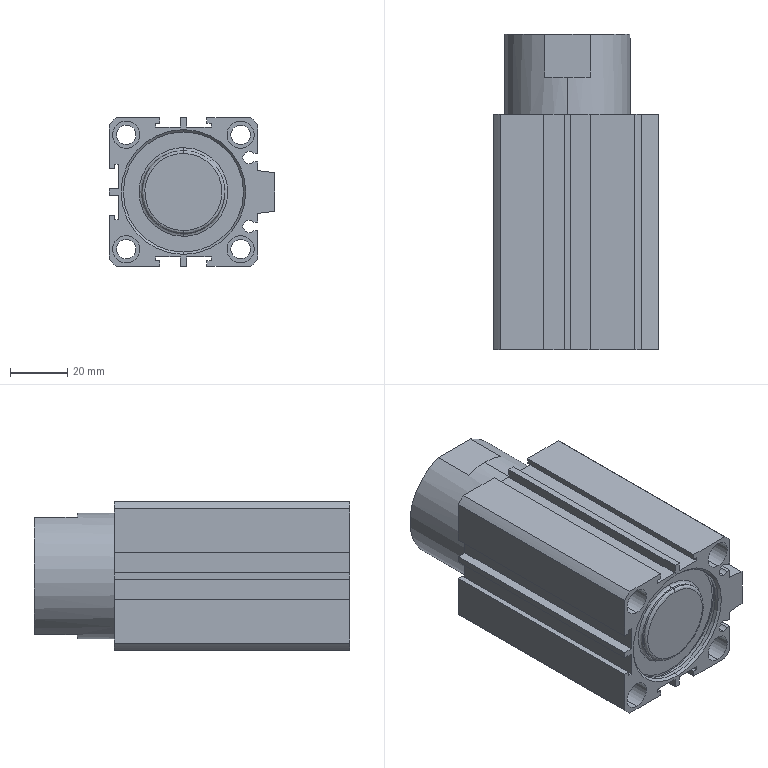Part | SolidWorks | features BaseBody 1 | 1 solid | 140 faces | box 58 x 110.2 x 52 mm | volume 147980 mm3 | plane 74 | cylinder 54 | cone 8 | spline 4 | commonest cylinder face diameters 9.5 x16 6.8 x8 4.4 x6 2.2 x4 42 x4 70 x4